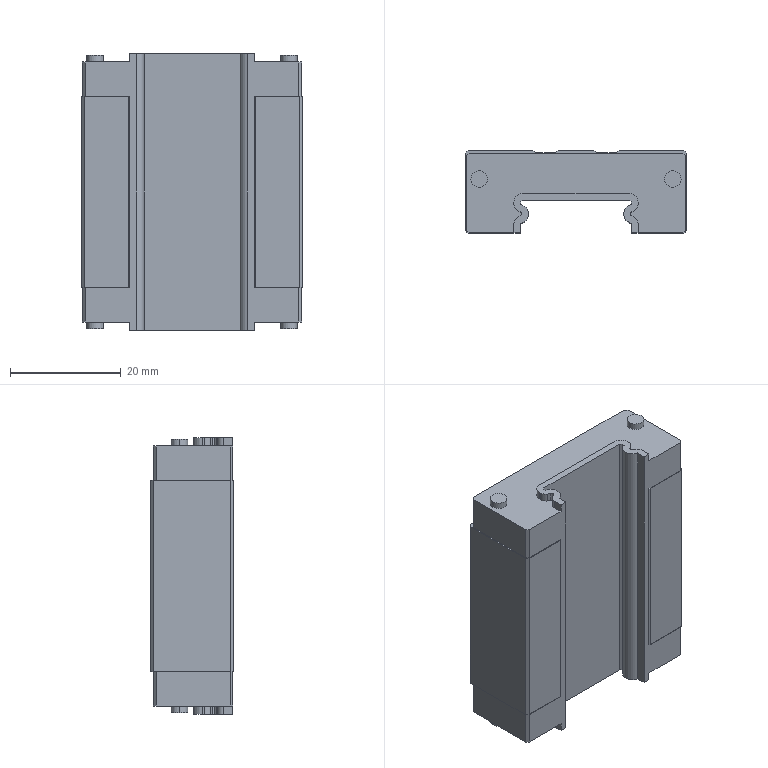Part | STEP file | b_SEZB20 | 1 solid | 123 faces | box 40 x 15 x 50 mm | volume 22286 mm3 | plane 70 | cylinder 37 | cone 16 | commonest cylinder face diameters 2.6 x8 3 x8 3.242 x8 0.8 x6 3.2 x4 3.529 x3